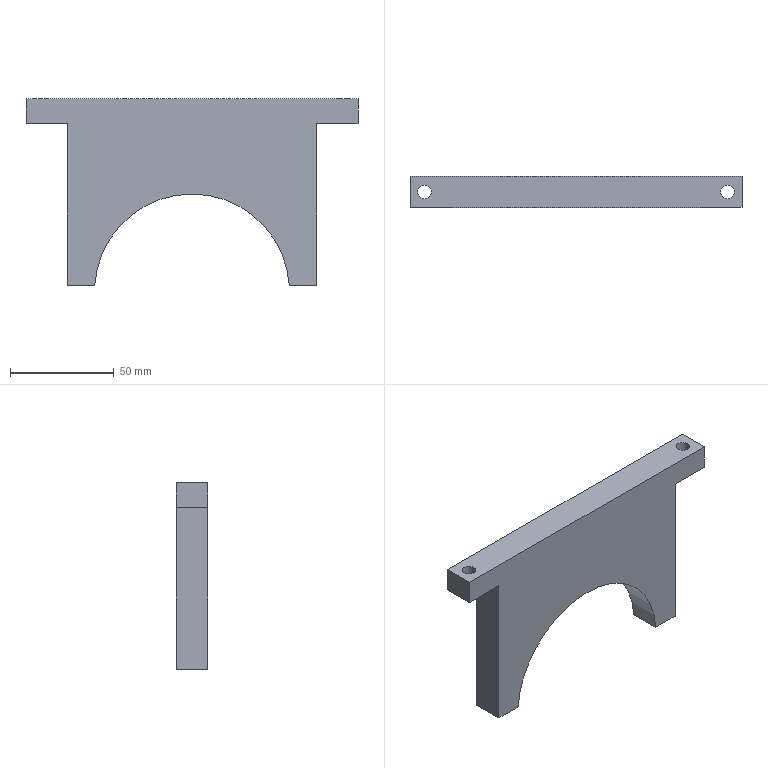Part | STEP file | 11-FG-S01511 | 1 solid | 24 faces | box 160 x 15 x 90 mm | volume 120227 mm3 | plane 11 | cylinder 9 | cone 4 | commonest cylinder face diameters 4.2 x4 6.5 x4 94 x1
STEP:
#1=CARTESIAN_POINT('',(-111.4,7.5,12.4));
#2=VERTEX_POINT('',#1);
#3=CARTESIAN_POINT('',(-115.6,7.5,12.4));
#4=VERTEX_POINT('',#3);
#5=CARTESIAN_POINT('',(-113.5,7.5,12.4));
#6=DIRECTION('',(0.,0.,-1.));
#7=DIRECTION('',(-1.,0.,0.));
#8=AXIS2_PLACEMENT_3D('',#5,#6,#7);
#9=CIRCLE('',#8,2.1);
#10=EDGE_CURVE('',#2,#4,#9,.T.);
#11=ORIENTED_EDGE('',*,*,#10,.F.);
#12=CARTESIAN_POINT('',(-111.4,7.5,0.));
#13=VERTEX_POINT('',#12);
#14=CARTESIAN_POINT('',(-111.4,7.5,0.));
#15=DIRECTION('',(0.,0.,-1.));
#16=VECTOR('',#15,1000.);
#17=LINE('',#14,#16);
#18=EDGE_CURVE('',#2,#13,#17,.T.);
#19=ORIENTED_EDGE('',*,*,#18,.T.);
#20=CARTESIAN_POINT('',(-115.6,7.5,0.));
#21=VERTEX_POINT('',#20);
#22=CARTESIAN_POINT('',(-113.5,7.5,0.));
#23=DIRECTION('',(0.,0.,-1.));
#24=DIRECTION('',(-1.,0.,0.));
#25=AXIS2_PLACEMENT_3D('',#22,#23,#24);
#26=CIRCLE('',#25,2.1);
#27=EDGE_CURVE('',#13,#21,#26,.T.);
#28=ORIENTED_EDGE('',*,*,#27,.T.);
#29=CARTESIAN_POINT('',(-115.6,7.5,0.));
#30=DIRECTION('',(0.,0.,-1.));
#31=VECTOR('',#30,1000.);
#32=LINE('',#29,#31);
#33=EDGE_CURVE('',#4,#21,#32,.T.);
#34=ORIENTED_EDGE('',*,*,#33,.F.);
#35=EDGE_LOOP('',(#11,#19,#28,#34));
#36=FACE_OUTER_BOUND('',#35,.T.);
#37=CARTESIAN_POINT('',(-113.5,7.5,0.));
#38=DIRECTION('',(0.,0.,-1.));
#39=DIRECTION('',(-1.,0.,0.));
#40=AXIS2_PLACEMENT_3D('',#37,#38,#39);
#41=CYLINDRICAL_SURFACE('',#40,2.1);
#42=ADVANCED_FACE('',(#36),#41,.F.);
#43=CARTESIAN_POINT('',(-113.5,7.5,13.662));
#44=VERTEX_POINT('',#43);
#45=CARTESIAN_POINT('',(-115.6,7.5,12.4));
#46=DIRECTION('',(-0.8572,0.,-0.515));
#47=VECTOR('',#46,1000.);
#48=LINE('',#45,#47);
#49=EDGE_CURVE('',#44,#4,#48,.T.);
#50=ORIENTED_EDGE('',*,*,#49,.F.);
#51=CARTESIAN_POINT('',(-111.4,7.5,12.4));
#52=DIRECTION('',(0.8572,0.,-0.515));
#53=VECTOR('',#52,1000.);
#54=LINE('',#51,#53);
#55=EDGE_CURVE('',#44,#2,#54,.T.);
#56=ORIENTED_EDGE('',*,*,#55,.T.);
#57=ORIENTED_EDGE('',*,*,#10,.T.);
#58=EDGE_LOOP('',(#50,#56,#57));
#59=FACE_OUTER_BOUND('',#58,.T.);
#60=CARTESIAN_POINT('',(-113.5,7.5,12.4));
#61=DIRECTION('',(0.,0.,-1.));
#62=DIRECTION('',(-1.,0.,0.));
#63=AXIS2_PLACEMENT_3D('',#60,#61,#62);
#64=CONICAL_SURFACE('',#63,2.1,1.03);
#65=ADVANCED_FACE('',(#59),#64,.F.);
#66=CARTESIAN_POINT('',(-4.4,7.5,12.4));
#67=VERTEX_POINT('',#66);
#68=CARTESIAN_POINT('',(-8.6,7.5,12.4));
#69=VERTEX_POINT('',#68);
#70=CARTESIAN_POINT('',(-6.5,7.5,12.4));
#71=DIRECTION('',(0.,0.,-1.));
#72=DIRECTION('',(-1.,0.,0.));
#73=AXIS2_PLACEMENT_3D('',#70,#71,#72);
#74=CIRCLE('',#73,2.1);
#75=EDGE_CURVE('',#67,#69,#74,.T.);
#76=ORIENTED_EDGE('',*,*,#75,.F.);
#77=CARTESIAN_POINT('',(-4.4,7.5,0.));
#78=VERTEX_POINT('',#77);
#79=CARTESIAN_POINT('',(-4.4,7.5,0.));
#80=DIRECTION('',(0.,0.,-1.));
#81=VECTOR('',#80,1000.);
#82=LINE('',#79,#81);
#83=EDGE_CURVE('',#67,#78,#82,.T.);
#84=ORIENTED_EDGE('',*,*,#83,.T.);
#85=CARTESIAN_POINT('',(-8.6,7.5,0.));
#86=VERTEX_POINT('',#85);
#87=CARTESIAN_POINT('',(-6.5,7.5,0.));
#88=DIRECTION('',(0.,0.,-1.));
#89=DIRECTION('',(-1.,0.,0.));
#90=AXIS2_PLACEMENT_3D('',#87,#88,#89);
#91=CIRCLE('',#90,2.1);
#92=EDGE_CURVE('',#78,#86,#91,.T.);
#93=ORIENTED_EDGE('',*,*,#92,.T.);
#94=CARTESIAN_POINT('',(-8.6,7.5,0.));
#95=DIRECTION('',(0.,0.,-1.));
#96=VECTOR('',#95,1000.);
#97=LINE('',#94,#96);
#98=EDGE_CURVE('',#69,#86,#97,.T.);
#99=ORIENTED_EDGE('',*,*,#98,.F.);
#100=EDGE_LOOP('',(#76,#84,#93,#99));
#101=FACE_OUTER_BOUND('',#100,.T.);
#102=CARTESIAN_POINT('',(-6.5,7.5,0.));
#103=DIRECTION('',(0.,0.,-1.));
#104=DIRECTION('',(-1.,0.,0.));
#105=AXIS2_PLACEMENT_3D('',#102,#103,#104);
#106=CYLINDRICAL_SURFACE('',#105,2.1);
#107=ADVANCED_FACE('',(#101),#106,.F.);
#108=CARTESIAN_POINT('',(-6.5,7.5,13.662));
#109=VERTEX_POINT('',#108);
#110=CARTESIAN_POINT('',(-8.6,7.5,12.4));
#111=DIRECTION('',(-0.8572,0.,-0.515));
#112=VECTOR('',#111,1000.);
#113=LINE('',#110,#112);
#114=EDGE_CURVE('',#109,#69,#113,.T.);
#115=ORIENTED_EDGE('',*,*,#114,.F.);
#116=CARTESIAN_POINT('',(-4.4,7.5,12.4));
#117=DIRECTION('',(0.8572,0.,-0.515));
#118=VECTOR('',#117,1000.);
#119=LINE('',#116,#118);
#120=EDGE_CURVE('',#109,#67,#119,.T.);
#121=ORIENTED_EDGE('',*,*,#120,.T.);
#122=ORIENTED_EDGE('',*,*,#75,.T.);
#123=EDGE_LOOP('',(#115,#121,#122));
#124=FACE_OUTER_BOUND('',#123,.T.);
#125=CARTESIAN_POINT('',(-6.5,7.5,12.4));
#126=DIRECTION('',(0.,0.,-1.));
#127=DIRECTION('',(-1.,0.,0.));
#128=AXIS2_PLACEMENT_3D('',#125,#126,#127);
#129=CONICAL_SURFACE('',#128,2.1,1.03);
#130=ADVANCED_FACE('',(#124),#129,.F.);
#131=CARTESIAN_POINT('',(-136.25,7.5,90.));
#132=VERTEX_POINT('',#131);
#133=CARTESIAN_POINT('',(-129.75,7.5,90.));
#134=VERTEX_POINT('',#133);
#135=CARTESIAN_POINT('',(-133.,7.5,90.));
#136=DIRECTION('',(0.,0.,1.));
#137=DIRECTION('',(1.,0.,0.));
#138=AXIS2_PLACEMENT_3D('',#135,#136,#137);
#139=CIRCLE('',#138,3.25);
#140=EDGE_CURVE('',#132,#134,#139,.T.);
#141=ORIENTED_EDGE('',*,*,#140,.T.);
#142=CARTESIAN_POINT('',(-129.75,7.5,78.));
#143=VERTEX_POINT('',#142);
#144=CARTESIAN_POINT('',(-129.75,7.5,158.));
#145=DIRECTION('',(0.,0.,-1.));
#146=VECTOR('',#145,1000.);
#147=LINE('',#144,#146);
#148=EDGE_CURVE('',#134,#143,#147,.T.);
#149=ORIENTED_EDGE('',*,*,#148,.T.);
#150=CARTESIAN_POINT('',(-136.25,7.5,78.));
#151=VERTEX_POINT('',#150);
#152=CARTESIAN_POINT('',(-133.,7.5,78.));
#153=DIRECTION('',(0.,0.,-1.));
#154=DIRECTION('',(1.,0.,0.));
#155=AXIS2_PLACEMENT_3D('',#152,#153,#154);
#156=CIRCLE('',#155,3.25);
#157=EDGE_CURVE('',#143,#151,#156,.T.);
#158=ORIENTED_EDGE('',*,*,#157,.T.);
#159=CARTESIAN_POINT('',(-136.25,7.5,158.));
#160=DIRECTION('',(0.,0.,-1.));
#161=VECTOR('',#160,1000.);
#162=LINE('',#159,#161);
#163=EDGE_CURVE('',#132,#151,#162,.T.);
#164=ORIENTED_EDGE('',*,*,#163,.F.);
#165=EDGE_LOOP('',(#141,#149,#158,#164));
#166=FACE_OUTER_BOUND('',#165,.T.);
#167=CARTESIAN_POINT('',(-133.,7.5,158.));
#168=DIRECTION('',(0.,0.,-1.));
#169=DIRECTION('',(-1.,0.,0.));
#170=AXIS2_PLACEMENT_3D('',#167,#168,#169);
#171=CYLINDRICAL_SURFACE('',#170,3.25);
#172=ADVANCED_FACE('',(#166),#171,.F.);
#173=CARTESIAN_POINT('',(9.75,7.5,90.));
#174=VERTEX_POINT('',#173);
#175=CARTESIAN_POINT('',(16.25,7.5,90.));
#176=VERTEX_POINT('',#175);
#177=CARTESIAN_POINT('',(13.,7.5,90.));
#178=DIRECTION('',(0.,0.,1.));
#179=DIRECTION('',(1.,0.,0.));
#180=AXIS2_PLACEMENT_3D('',#177,#178,#179);
#181=CIRCLE('',#180,3.25);
#182=EDGE_CURVE('',#174,#176,#181,.T.);
#183=ORIENTED_EDGE('',*,*,#182,.T.);
#184=CARTESIAN_POINT('',(16.25,7.5,78.));
#185=VERTEX_POINT('',#184);
#186=CARTESIAN_POINT('',(16.25,7.5,158.));
#187=DIRECTION('',(0.,0.,-1.));
#188=VECTOR('',#187,1000.);
#189=LINE('',#186,#188);
#190=EDGE_CURVE('',#176,#185,#189,.T.);
#191=ORIENTED_EDGE('',*,*,#190,.T.);
#192=CARTESIAN_POINT('',(9.75,7.5,78.));
#193=VERTEX_POINT('',#192);
#194=CARTESIAN_POINT('',(13.,7.5,78.));
#195=DIRECTION('',(0.,0.,-1.));
#196=DIRECTION('',(-1.,0.,0.));
#197=AXIS2_PLACEMENT_3D('',#194,#195,#196);
#198=CIRCLE('',#197,3.25);
#199=EDGE_CURVE('',#185,#193,#198,.T.);
#200=ORIENTED_EDGE('',*,*,#199,.T.);
#201=CARTESIAN_POINT('',(9.75,7.5,158.));
#202=DIRECTION('',(0.,0.,-1.));
#203=VECTOR('',#202,1000.);
#204=LINE('',#201,#203);
#205=EDGE_CURVE('',#174,#193,#204,.T.);
#206=ORIENTED_EDGE('',*,*,#205,.F.);
#207=EDGE_LOOP('',(#183,#191,#200,#206));
#208=FACE_OUTER_BOUND('',#207,.T.);
#209=CARTESIAN_POINT('',(13.,7.5,158.));
#210=DIRECTION('',(0.,0.,-1.));
#211=DIRECTION('',(-1.,0.,0.));
#212=AXIS2_PLACEMENT_3D('',#209,#210,#211);
#213=CYLINDRICAL_SURFACE('',#212,3.25);
#214=ADVANCED_FACE('',(#208),#213,.F.);
#215=CARTESIAN_POINT('',(-120.,15.,78.));
#216=VERTEX_POINT('',#215);
#217=CARTESIAN_POINT('',(-120.,0.,78.));
#218=VERTEX_POINT('',#217);
#219=CARTESIAN_POINT('',(-120.,38.324,78.));
#220=DIRECTION('',(0.,-1.,0.));
#221=VECTOR('',#220,1000.);
#222=LINE('',#219,#221);
#223=EDGE_CURVE('',#216,#218,#222,.T.);
#224=ORIENTED_EDGE('',*,*,#223,.F.);
#225=CARTESIAN_POINT('',(-120.,15.,0.));
#226=VERTEX_POINT('',#225);
#227=CARTESIAN_POINT('',(-120.,15.,90.));
#228=DIRECTION('',(0.,0.,-1.));
#229=VECTOR('',#228,1000.);
#230=LINE('',#227,#229);
#231=EDGE_CURVE('',#216,#226,#230,.T.);
#232=ORIENTED_EDGE('',*,*,#231,.T.);
#233=CARTESIAN_POINT('',(-120.,0.,0.));
#234=VERTEX_POINT('',#233);
#235=CARTESIAN_POINT('',(-120.,0.,0.));
#236=DIRECTION('',(0.,-1.,0.));
#237=VECTOR('',#236,1000.);
#238=LINE('',#235,#237);
#239=EDGE_CURVE('',#226,#234,#238,.T.);
#240=ORIENTED_EDGE('',*,*,#239,.T.);
#241=CARTESIAN_POINT('',(-120.,0.,90.));
#242=DIRECTION('',(0.,0.,-1.));
#243=VECTOR('',#242,1000.);
#244=LINE('',#241,#243);
#245=EDGE_CURVE('',#218,#234,#244,.T.);
#246=ORIENTED_EDGE('',*,*,#245,.F.);
#247=EDGE_LOOP('',(#224,#232,#240,#246));
#248=FACE_OUTER_BOUND('',#247,.T.);
#249=CARTESIAN_POINT('',(-120.,0.,90.));
#250=DIRECTION('',(1.,0.,0.));
#251=DIRECTION('',(0.,0.,-1.));
#252=AXIS2_PLACEMENT_3D('',#249,#250,#251);
#253=PLANE('',#252);
#254=ADVANCED_FACE('',(#248),#253,.F.);
#255=CARTESIAN_POINT('',(-113.5,7.5,0.));
#256=DIRECTION('',(0.,0.,-1.));
#257=DIRECTION('',(-1.,0.,0.));
#258=AXIS2_PLACEMENT_3D('',#255,#256,#257);
#259=CIRCLE('',#258,2.1);
#260=EDGE_CURVE('',#21,#13,#259,.T.);
#261=ORIENTED_EDGE('',*,*,#260,.F.);
#262=ORIENTED_EDGE('',*,*,#27,.F.);
#263=EDGE_LOOP('',(#261,#262));
#264=FACE_BOUND('',#263,.T.);
#265=CARTESIAN_POINT('',(-106.904,15.,0.));
#266=VERTEX_POINT('',#265);
#267=CARTESIAN_POINT('',(0.,15.,0.));
#268=DIRECTION('',(-1.,0.,0.));
#269=VECTOR('',#268,1000.);
#270=LINE('',#267,#269);
#271=EDGE_CURVE('',#266,#226,#270,.T.);
#272=ORIENTED_EDGE('',*,*,#271,.F.);
#273=CARTESIAN_POINT('',(-106.904,0.,0.));
#274=VERTEX_POINT('',#273);
#275=CARTESIAN_POINT('',(-106.904,80.,0.));
#276=DIRECTION('',(0.,-1.,0.));
#277=VECTOR('',#276,1000.);
#278=LINE('',#275,#277);
#279=EDGE_CURVE('',#266,#274,#278,.T.);
#280=ORIENTED_EDGE('',*,*,#279,.T.);
#281=CARTESIAN_POINT('',(0.,0.,0.));
#282=DIRECTION('',(1.,0.,0.));
#283=VECTOR('',#282,1000.);
#284=LINE('',#281,#283);
#285=EDGE_CURVE('',#234,#274,#284,.T.);
#286=ORIENTED_EDGE('',*,*,#285,.F.);
#287=ORIENTED_EDGE('',*,*,#239,.F.);
#288=EDGE_LOOP('',(#272,#280,#286,#287));
#289=FACE_OUTER_BOUND('',#288,.T.);
#290=CARTESIAN_POINT('',(0.,15.,0.));
#291=DIRECTION('',(0.,0.,1.));
#292=DIRECTION('',(1.,0.,0.));
#293=AXIS2_PLACEMENT_3D('',#290,#291,#292);
#294=PLANE('',#293);
#295=ADVANCED_FACE('',(#264,#289),#294,.F.);
#296=CARTESIAN_POINT('',(0.,15.,78.));
#297=VERTEX_POINT('',#296);
#298=CARTESIAN_POINT('',(0.,15.,0.));
#299=VERTEX_POINT('',#298);
#300=CARTESIAN_POINT('',(0.,15.,90.));
#301=DIRECTION('',(0.,0.,-1.));
#302=VECTOR('',#301,1000.);
#303=LINE('',#300,#302);
#304=EDGE_CURVE('',#297,#299,#303,.T.);
#305=ORIENTED_EDGE('',*,*,#304,.F.);
#306=CARTESIAN_POINT('',(0.,0.,78.));
#307=VERTEX_POINT('',#306);
#308=CARTESIAN_POINT('',(0.,38.324,78.));
#309=DIRECTION('',(0.,-1.,0.));
#310=VECTOR('',#309,1000.);
#311=LINE('',#308,#310);
#312=EDGE_CURVE('',#297,#307,#311,.T.);
#313=ORIENTED_EDGE('',*,*,#312,.T.);
#314=CARTESIAN_POINT('',(0.,0.,0.));
#315=VERTEX_POINT('',#314);
#316=CARTESIAN_POINT('',(0.,0.,90.));
#317=DIRECTION('',(0.,0.,-1.));
#318=VECTOR('',#317,1000.);
#319=LINE('',#316,#318);
#320=EDGE_CURVE('',#307,#315,#319,.T.);
#321=ORIENTED_EDGE('',*,*,#320,.T.);
#322=CARTESIAN_POINT('',(0.,0.,0.));
#323=DIRECTION('',(0.,1.,0.));
#324=VECTOR('',#323,1000.);
#325=LINE('',#322,#324);
#326=EDGE_CURVE('',#315,#299,#325,.T.);
#327=ORIENTED_EDGE('',*,*,#326,.T.);
#328=EDGE_LOOP('',(#305,#313,#321,#327));
#329=FACE_OUTER_BOUND('',#328,.T.);
#330=CARTESIAN_POINT('',(0.,0.,90.));
#331=DIRECTION('',(-1.,0.,0.));
#332=DIRECTION('',(0.,0.,1.));
#333=AXIS2_PLACEMENT_3D('',#330,#331,#332);
#334=PLANE('',#333);
#335=ADVANCED_FACE('',(#329),#334,.F.);
#336=CARTESIAN_POINT('',(-13.096,15.,0.));
#337=VERTEX_POINT('',#336);
#338=CARTESIAN_POINT('',(0.,15.,0.));
#339=DIRECTION('',(-1.,0.,0.));
#340=VECTOR('',#339,1000.);
#341=LINE('',#338,#340);
#342=EDGE_CURVE('',#299,#337,#341,.T.);
#343=ORIENTED_EDGE('',*,*,#342,.T.);
#344=CARTESIAN_POINT('',(-60.,15.,-3.));
#345=DIRECTION('',(0.,-1.,0.));
#346=DIRECTION('',(1.,0.,0.));
#347=AXIS2_PLACEMENT_3D('',#344,#345,#346);
#348=CIRCLE('',#347,47.);
#349=EDGE_CURVE('',#337,#266,#348,.T.);
#350=ORIENTED_EDGE('',*,*,#349,.T.);
#351=ORIENTED_EDGE('',*,*,#271,.T.);
#352=ORIENTED_EDGE('',*,*,#231,.F.);
#353=CARTESIAN_POINT('',(-140.,15.,78.));
#354=VERTEX_POINT('',#353);
#355=CARTESIAN_POINT('',(-120.,15.,78.));
#356=DIRECTION('',(-1.,0.,0.));
#357=VECTOR('',#356,1000.);
#358=LINE('',#355,#357);
#359=EDGE_CURVE('',#216,#354,#358,.T.);
#360=ORIENTED_EDGE('',*,*,#359,.T.);
#361=CARTESIAN_POINT('',(-140.,15.,90.));
#362=VERTEX_POINT('',#361);
#363=CARTESIAN_POINT('',(-140.,15.,90.));
#364=DIRECTION('',(0.,0.,1.));
#365=VECTOR('',#364,1000.);
#366=LINE('',#363,#365);
#367=EDGE_CURVE('',#354,#362,#366,.T.);
#368=ORIENTED_EDGE('',*,*,#367,.T.);
#369=CARTESIAN_POINT('',(20.,15.,90.));
#370=VERTEX_POINT('',#369);
#371=CARTESIAN_POINT('',(0.,15.,90.));
#372=DIRECTION('',(-1.,0.,0.));
#373=VECTOR('',#372,1000.);
#374=LINE('',#371,#373);
#375=EDGE_CURVE('',#370,#362,#374,.T.);
#376=ORIENTED_EDGE('',*,*,#375,.F.);
#377=CARTESIAN_POINT('',(20.,15.,78.));
#378=VERTEX_POINT('',#377);
#379=CARTESIAN_POINT('',(20.,15.,90.));
#380=DIRECTION('',(0.,0.,-1.));
#381=VECTOR('',#380,1000.);
#382=LINE('',#379,#381);
#383=EDGE_CURVE('',#370,#378,#382,.T.);
#384=ORIENTED_EDGE('',*,*,#383,.T.);
#385=CARTESIAN_POINT('',(0.,15.,78.));
#386=DIRECTION('',(-1.,0.,0.));
#387=VECTOR('',#386,1000.);
#388=LINE('',#385,#387);
#389=EDGE_CURVE('',#378,#297,#388,.T.);
#390=ORIENTED_EDGE('',*,*,#389,.T.);
#391=ORIENTED_EDGE('',*,*,#304,.T.);
#392=EDGE_LOOP('',(#343,#350,#351,#352,#360,#368,#376,#384,#390,#391));
#393=FACE_OUTER_BOUND('',#392,.T.);
#394=CARTESIAN_POINT('',(0.,15.,90.));
#395=DIRECTION('',(0.,-1.,0.));
#396=DIRECTION('',(1.,0.,0.));
#397=AXIS2_PLACEMENT_3D('',#394,#395,#396);
#398=PLANE('',#397);
#399=ADVANCED_FACE('',(#393),#398,.F.);
#400=ORIENTED_EDGE('',*,*,#285,.T.);
#401=CARTESIAN_POINT('',(-13.096,0.,0.));
#402=VERTEX_POINT('',#401);
#403=CARTESIAN_POINT('',(-60.,0.,-3.));
#404=DIRECTION('',(0.,-1.,0.));
#405=DIRECTION('',(1.,0.,0.));
#406=AXIS2_PLACEMENT_3D('',#403,#404,#405);
#407=CIRCLE('',#406,47.);
#408=EDGE_CURVE('',#402,#274,#407,.T.);
#409=ORIENTED_EDGE('',*,*,#408,.F.);
#410=CARTESIAN_POINT('',(0.,0.,0.));
#411=DIRECTION('',(1.,0.,0.));
#412=VECTOR('',#411,1000.);
#413=LINE('',#410,#412);
#414=EDGE_CURVE('',#402,#315,#413,.T.);
#415=ORIENTED_EDGE('',*,*,#414,.T.);
#416=ORIENTED_EDGE('',*,*,#320,.F.);
#417=CARTESIAN_POINT('',(20.,0.,78.));
#418=VERTEX_POINT('',#417);
#419=CARTESIAN_POINT('',(0.,0.,78.));
#420=DIRECTION('',(1.,0.,0.));
#421=VECTOR('',#420,1000.);
#422=LINE('',#419,#421);
#423=EDGE_CURVE('',#307,#418,#422,.T.);
#424=ORIENTED_EDGE('',*,*,#423,.T.);
#425=CARTESIAN_POINT('',(20.,0.,90.));
#426=VERTEX_POINT('',#425);
#427=CARTESIAN_POINT('',(20.,0.,90.));
#428=DIRECTION('',(0.,0.,1.));
#429=VECTOR('',#428,1000.);
#430=LINE('',#427,#429);
#431=EDGE_CURVE('',#418,#426,#430,.T.);
#432=ORIENTED_EDGE('',*,*,#431,.T.);
#433=CARTESIAN_POINT('',(-140.,0.,90.));
#434=VERTEX_POINT('',#433);
#435=CARTESIAN_POINT('',(0.,0.,90.));
#436=DIRECTION('',(1.,0.,0.));
#437=VECTOR('',#436,1000.);
#438=LINE('',#435,#437);
#439=EDGE_CURVE('',#434,#426,#438,.T.);
#440=ORIENTED_EDGE('',*,*,#439,.F.);
#441=CARTESIAN_POINT('',(-140.,0.,78.));
#442=VERTEX_POINT('',#441);
#443=CARTESIAN_POINT('',(-140.,0.,90.));
#444=DIRECTION('',(0.,0.,-1.));
#445=VECTOR('',#444,1000.);
#446=LINE('',#443,#445);
#447=EDGE_CURVE('',#434,#442,#446,.T.);
#448=ORIENTED_EDGE('',*,*,#447,.T.);
#449=CARTESIAN_POINT('',(-120.,0.,78.));
#450=DIRECTION('',(1.,0.,0.));
#451=VECTOR('',#450,1000.);
#452=LINE('',#449,#451);
#453=EDGE_CURVE('',#442,#218,#452,.T.);
#454=ORIENTED_EDGE('',*,*,#453,.T.);
#455=ORIENTED_EDGE('',*,*,#245,.T.);
#456=EDGE_LOOP('',(#400,#409,#415,#416,#424,#432,#440,#448,#454,#455));
#457=FACE_OUTER_BOUND('',#456,.T.);
#458=CARTESIAN_POINT('',(0.,0.,90.));
#459=DIRECTION('',(0.,1.,0.));
#460=DIRECTION('',(-1.,0.,0.));
#461=AXIS2_PLACEMENT_3D('',#458,#459,#460);
#462=PLANE('',#461);
#463=ADVANCED_FACE('',(#457),#462,.F.);
#464=ORIENTED_EDGE('',*,*,#140,.F.);
#465=CARTESIAN_POINT('',(-133.,7.5,90.));
#466=DIRECTION('',(0.,0.,1.));
#467=DIRECTION('',(1.,0.,0.));
#468=AXIS2_PLACEMENT_3D('',#465,#466,#467);
#469=CIRCLE('',#468,3.25);
#470=EDGE_CURVE('',#134,#132,#469,.T.);
#471=ORIENTED_EDGE('',*,*,#470,.F.);
#472=EDGE_LOOP('',(#464,#471));
#473=FACE_BOUND('',#472,.T.);
#474=ORIENTED_EDGE('',*,*,#182,.F.);
#475=CARTESIAN_POINT('',(13.,7.5,90.));
#476=DIRECTION('',(0.,0.,1.));
#477=DIRECTION('',(1.,0.,0.));
#478=AXIS2_PLACEMENT_3D('',#475,#476,#477);
#479=CIRCLE('',#478,3.25);
#480=EDGE_CURVE('',#176,#174,#479,.T.);
#481=ORIENTED_EDGE('',*,*,#480,.F.);
#482=EDGE_LOOP('',(#474,#481));
#483=FACE_BOUND('',#482,.T.);
#484=ORIENTED_EDGE('',*,*,#439,.T.);
#485=CARTESIAN_POINT('',(20.,38.324,90.));
#486=DIRECTION('',(0.,-1.,0.));
#487=VECTOR('',#486,1000.);
#488=LINE('',#485,#487);
#489=EDGE_CURVE('',#370,#426,#488,.T.);
#490=ORIENTED_EDGE('',*,*,#489,.F.);
#491=ORIENTED_EDGE('',*,*,#375,.T.);
#492=CARTESIAN_POINT('',(-140.,38.324,90.));
#493=DIRECTION('',(0.,-1.,0.));
#494=VECTOR('',#493,1000.);
#495=LINE('',#492,#494);
#496=EDGE_CURVE('',#362,#434,#495,.T.);
#497=ORIENTED_EDGE('',*,*,#496,.T.);
#498=EDGE_LOOP('',(#484,#490,#491,#497));
#499=FACE_OUTER_BOUND('',#498,.T.);
#500=CARTESIAN_POINT('',(0.,15.,90.));
#501=DIRECTION('',(0.,0.,1.));
#502=DIRECTION('',(1.,0.,0.));
#503=AXIS2_PLACEMENT_3D('',#500,#501,#502);
#504=PLANE('',#503);
#505=ADVANCED_FACE('',(#473,#483,#499),#504,.T.);
#506=CARTESIAN_POINT('',(-6.5,7.5,0.));
#507=DIRECTION('',(0.,0.,-1.));
#508=DIRECTION('',(-1.,0.,0.));
#509=AXIS2_PLACEMENT_3D('',#506,#507,#508);
#510=CIRCLE('',#509,2.1);
#511=EDGE_CURVE('',#86,#78,#510,.T.);
#512=ORIENTED_EDGE('',*,*,#511,.F.);
#513=ORIENTED_EDGE('',*,*,#92,.F.);
#514=EDGE_LOOP('',(#512,#513));
#515=FACE_BOUND('',#514,.T.);
#516=ORIENTED_EDGE('',*,*,#414,.F.);
#517=CARTESIAN_POINT('',(-13.096,80.,0.));
#518=DIRECTION('',(0.,1.,0.));
#519=VECTOR('',#518,1000.);
#520=LINE('',#517,#519);
#521=EDGE_CURVE('',#402,#337,#520,.T.);
#522=ORIENTED_EDGE('',*,*,#521,.T.);
#523=ORIENTED_EDGE('',*,*,#342,.F.);
#524=ORIENTED_EDGE('',*,*,#326,.F.);
#525=EDGE_LOOP('',(#516,#522,#523,#524));
#526=FACE_OUTER_BOUND('',#525,.T.);
#527=CARTESIAN_POINT('',(0.,15.,0.));
#528=DIRECTION('',(0.,0.,1.));
#529=DIRECTION('',(1.,0.,0.));
#530=AXIS2_PLACEMENT_3D('',#527,#528,#529);
#531=PLANE('',#530);
#532=ADVANCED_FACE('',(#515,#526),#531,.F.);
#533=ORIENTED_EDGE('',*,*,#349,.F.);
#534=ORIENTED_EDGE('',*,*,#521,.F.);
#535=ORIENTED_EDGE('',*,*,#408,.T.);
#536=ORIENTED_EDGE('',*,*,#279,.F.);
#537=EDGE_LOOP('',(#533,#534,#535,#536));
#538=FACE_OUTER_BOUND('',#537,.T.);
#539=CARTESIAN_POINT('',(-60.,80.,-3.));
#540=DIRECTION('',(0.,-1.,0.));
#541=DIRECTION('',(1.,0.,0.));
#542=AXIS2_PLACEMENT_3D('',#539,#540,#541);
#543=CYLINDRICAL_SURFACE('',#542,47.);
#544=ADVANCED_FACE('',(#538),#543,.F.);
#545=CARTESIAN_POINT('',(-133.,7.5,78.));
#546=DIRECTION('',(0.,0.,-1.));
#547=DIRECTION('',(1.,0.,0.));
#548=AXIS2_PLACEMENT_3D('',#545,#546,#547);
#549=CIRCLE('',#548,3.25);
#550=EDGE_CURVE('',#151,#143,#549,.T.);
#551=ORIENTED_EDGE('',*,*,#550,.F.);
#552=ORIENTED_EDGE('',*,*,#157,.F.);
#553=EDGE_LOOP('',(#551,#552));
#554=FACE_BOUND('',#553,.T.);
#555=ORIENTED_EDGE('',*,*,#359,.F.);
#556=ORIENTED_EDGE('',*,*,#223,.T.);
#557=ORIENTED_EDGE('',*,*,#453,.F.);
#558=CARTESIAN_POINT('',(-140.,38.324,78.));
#559=DIRECTION('',(0.,-1.,0.));
#560=VECTOR('',#559,1000.);
#561=LINE('',#558,#560);
#562=EDGE_CURVE('',#354,#442,#561,.T.);
#563=ORIENTED_EDGE('',*,*,#562,.F.);
#564=EDGE_LOOP('',(#555,#556,#557,#563));
#565=FACE_OUTER_BOUND('',#564,.T.);
#566=CARTESIAN_POINT('',(-120.,38.324,78.));
#567=DIRECTION('',(0.,0.,-1.));
#568=DIRECTION('',(-1.,0.,0.));
#569=AXIS2_PLACEMENT_3D('',#566,#567,#568);
#570=PLANE('',#569);
#571=ADVANCED_FACE('',(#554,#565),#570,.T.);
#572=ORIENTED_EDGE('',*,*,#367,.F.);
#573=ORIENTED_EDGE('',*,*,#562,.T.);
#574=ORIENTED_EDGE('',*,*,#447,.F.);
#575=ORIENTED_EDGE('',*,*,#496,.F.);
#576=EDGE_LOOP('',(#572,#573,#574,#575));
#577=FACE_OUTER_BOUND('',#576,.T.);
#578=CARTESIAN_POINT('',(-140.,38.324,90.));
#579=DIRECTION('',(-1.,0.,0.));
#580=DIRECTION('',(0.,0.,1.));
#581=AXIS2_PLACEMENT_3D('',#578,#579,#580);
#582=PLANE('',#581);
#583=ADVANCED_FACE('',(#577),#582,.T.);
#584=ORIENTED_EDGE('',*,*,#383,.F.);
#585=ORIENTED_EDGE('',*,*,#489,.T.);
#586=ORIENTED_EDGE('',*,*,#431,.F.);
#587=CARTESIAN_POINT('',(20.,38.324,78.));
#588=DIRECTION('',(0.,-1.,0.));
#589=VECTOR('',#588,1000.);
#590=LINE('',#587,#589);
#591=EDGE_CURVE('',#378,#418,#590,.T.);
#592=ORIENTED_EDGE('',*,*,#591,.F.);
#593=EDGE_LOOP('',(#584,#585,#586,#592));
#594=FACE_OUTER_BOUND('',#593,.T.);
#595=CARTESIAN_POINT('',(20.,38.324,90.));
#596=DIRECTION('',(1.,0.,0.));
#597=DIRECTION('',(0.,1.,0.));
#598=AXIS2_PLACEMENT_3D('',#595,#596,#597);
#599=PLANE('',#598);
#600=ADVANCED_FACE('',(#594),#599,.T.);
#601=CARTESIAN_POINT('',(13.,7.5,78.));
#602=DIRECTION('',(0.,0.,-1.));
#603=DIRECTION('',(-1.,0.,0.));
#604=AXIS2_PLACEMENT_3D('',#601,#602,#603);
#605=CIRCLE('',#604,3.25);
#606=EDGE_CURVE('',#193,#185,#605,.T.);
#607=ORIENTED_EDGE('',*,*,#606,.F.);
#608=ORIENTED_EDGE('',*,*,#199,.F.);
#609=EDGE_LOOP('',(#607,#608));
#610=FACE_BOUND('',#609,.T.);
#611=ORIENTED_EDGE('',*,*,#389,.F.);
#612=ORIENTED_EDGE('',*,*,#591,.T.);
#613=ORIENTED_EDGE('',*,*,#423,.F.);
#614=ORIENTED_EDGE('',*,*,#312,.F.);
#615=EDGE_LOOP('',(#611,#612,#613,#614));
#616=FACE_OUTER_BOUND('',#615,.T.);
#617=CARTESIAN_POINT('',(0.,38.324,78.));
#618=DIRECTION('',(0.,0.,-1.));
#619=DIRECTION('',(-1.,0.,0.));
#620=AXIS2_PLACEMENT_3D('',#617,#618,#619);
#621=PLANE('',#620);
#622=ADVANCED_FACE('',(#610,#616),#621,.T.);
#623=ORIENTED_EDGE('',*,*,#190,.F.);
#624=ORIENTED_EDGE('',*,*,#480,.T.);
#625=ORIENTED_EDGE('',*,*,#205,.T.);
#626=ORIENTED_EDGE('',*,*,#606,.T.);
#627=EDGE_LOOP('',(#623,#624,#625,#626));
#628=FACE_OUTER_BOUND('',#627,.T.);
#629=CARTESIAN_POINT('',(13.,7.5,158.));
#630=DIRECTION('',(0.,0.,-1.));
#631=DIRECTION('',(-1.,0.,0.));
#632=AXIS2_PLACEMENT_3D('',#629,#630,#631);
#633=CYLINDRICAL_SURFACE('',#632,3.25);
#634=ADVANCED_FACE('',(#628),#633,.F.);
#635=ORIENTED_EDGE('',*,*,#148,.F.);
#636=ORIENTED_EDGE('',*,*,#470,.T.);
#637=ORIENTED_EDGE('',*,*,#163,.T.);
#638=ORIENTED_EDGE('',*,*,#550,.T.);
#639=EDGE_LOOP('',(#635,#636,#637,#638));
#640=FACE_OUTER_BOUND('',#639,.T.);
#641=CARTESIAN_POINT('',(-133.,7.5,158.));
#642=DIRECTION('',(0.,0.,-1.));
#643=DIRECTION('',(-1.,0.,0.));
#644=AXIS2_PLACEMENT_3D('',#641,#642,#643);
#645=CYLINDRICAL_SURFACE('',#644,3.25);
#646=ADVANCED_FACE('',(#640),#645,.F.);
#647=ORIENTED_EDGE('',*,*,#120,.F.);
#648=ORIENTED_EDGE('',*,*,#114,.T.);
#649=CARTESIAN_POINT('',(-6.5,7.5,12.4));
#650=DIRECTION('',(0.,0.,-1.));
#651=DIRECTION('',(-1.,0.,0.));
#652=AXIS2_PLACEMENT_3D('',#649,#650,#651);
#653=CIRCLE('',#652,2.1);
#654=EDGE_CURVE('',#69,#67,#653,.T.);
#655=ORIENTED_EDGE('',*,*,#654,.T.);
#656=EDGE_LOOP('',(#647,#648,#655));
#657=FACE_OUTER_BOUND('',#656,.T.);
#658=CARTESIAN_POINT('',(-6.5,7.5,12.4));
#659=DIRECTION('',(0.,0.,-1.));
#660=DIRECTION('',(-1.,0.,0.));
#661=AXIS2_PLACEMENT_3D('',#658,#659,#660);
#662=CONICAL_SURFACE('',#661,2.1,1.03);
#663=ADVANCED_FACE('',(#657),#662,.F.);
#664=ORIENTED_EDGE('',*,*,#83,.F.);
#665=ORIENTED_EDGE('',*,*,#654,.F.);
#666=ORIENTED_EDGE('',*,*,#98,.T.);
#667=ORIENTED_EDGE('',*,*,#511,.T.);
#668=EDGE_LOOP('',(#664,#665,#666,#667));
#669=FACE_OUTER_BOUND('',#668,.T.);
#670=CARTESIAN_POINT('',(-6.5,7.5,0.));
#671=DIRECTION('',(0.,0.,-1.));
#672=DIRECTION('',(-1.,0.,0.));
#673=AXIS2_PLACEMENT_3D('',#670,#671,#672);
#674=CYLINDRICAL_SURFACE('',#673,2.1);
#675=ADVANCED_FACE('',(#669),#674,.F.);
#676=ORIENTED_EDGE('',*,*,#55,.F.);
#677=ORIENTED_EDGE('',*,*,#49,.T.);
#678=CARTESIAN_POINT('',(-113.5,7.5,12.4));
#679=DIRECTION('',(0.,0.,-1.));
#680=DIRECTION('',(-1.,0.,0.));
#681=AXIS2_PLACEMENT_3D('',#678,#679,#680);
#682=CIRCLE('',#681,2.1);
#683=EDGE_CURVE('',#4,#2,#682,.T.);
#684=ORIENTED_EDGE('',*,*,#683,.T.);
#685=EDGE_LOOP('',(#676,#677,#684));
#686=FACE_OUTER_BOUND('',#685,.T.);
#687=CARTESIAN_POINT('',(-113.5,7.5,12.4));
#688=DIRECTION('',(0.,0.,-1.));
#689=DIRECTION('',(-1.,0.,0.));
#690=AXIS2_PLACEMENT_3D('',#687,#688,#689);
#691=CONICAL_SURFACE('',#690,2.1,1.03);
#692=ADVANCED_FACE('',(#686),#691,.F.);
#693=ORIENTED_EDGE('',*,*,#18,.F.);
#694=ORIENTED_EDGE('',*,*,#683,.F.);
#695=ORIENTED_EDGE('',*,*,#33,.T.);
#696=ORIENTED_EDGE('',*,*,#260,.T.);
#697=EDGE_LOOP('',(#693,#694,#695,#696));
#698=FACE_OUTER_BOUND('',#697,.T.);
#699=CARTESIAN_POINT('',(-113.5,7.5,0.));
#700=DIRECTION('',(0.,0.,-1.));
#701=DIRECTION('',(-1.,0.,0.));
#702=AXIS2_PLACEMENT_3D('',#699,#700,#701);
#703=CYLINDRICAL_SURFACE('',#702,2.1);
#704=ADVANCED_FACE('',(#698),#703,.F.);
#705=CLOSED_SHELL('',(#42,#65,#107,#130,#172,#214,#254,#295,#335,#399,#463,#505,#532,#544,#571,#583,#600,#622,#634,#646,#663,#675,#692,#704));
#706=MANIFOLD_SOLID_BREP('',#705);
#707=CARTESIAN_POINT('',(0.,0.,0.));
#708=DIRECTION('',(0.,0.,1.));
#709=DIRECTION('',(1.,0.,0.));
#710=AXIS2_PLACEMENT_3D('',#707,#708,#709);
#711=(LENGTH_UNIT()NAMED_UNIT(*)SI_UNIT(.MILLI.,.METRE.));
#712=UNCERTAINTY_MEASURE_WITH_UNIT(LENGTH_MEASURE(0.00001),#711,'','');
#713=(NAMED_UNIT(*)PLANE_ANGLE_UNIT()SI_UNIT($,.RADIAN.));
#714=(NAMED_UNIT(*)SI_UNIT($,.STERADIAN.)SOLID_ANGLE_UNIT());
#715=(GEOMETRIC_REPRESENTATION_CONTEXT(3)GLOBAL_UNCERTAINTY_ASSIGNED_CONTEXT((#712))GLOBAL_UNIT_ASSIGNED_CONTEXT((#711,#713,#714))REPRESENTATION_CONTEXT('',''));
#716=ADVANCED_BREP_SHAPE_REPRESENTATION('',(#706,#710),#715);